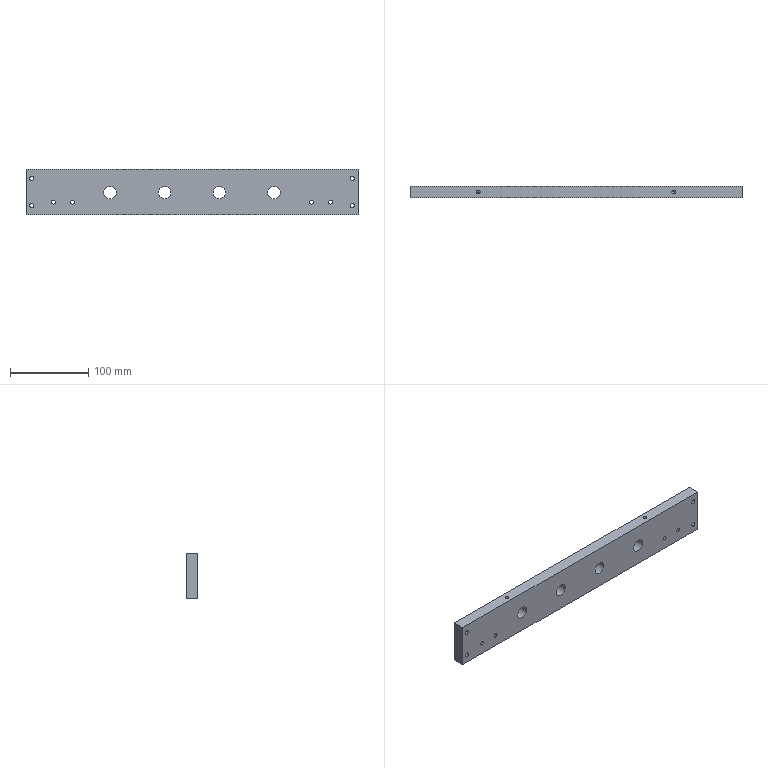Part | STEP file | Front side plate B | 1 solid | 50 faces | box 425 x 15 x 58 mm | volume 353146 mm3 | cylinder 36 | plane 10 | cone 4 | commonest cylinder face diameters 5 x12 5.5 x8 10 x8 16 x8